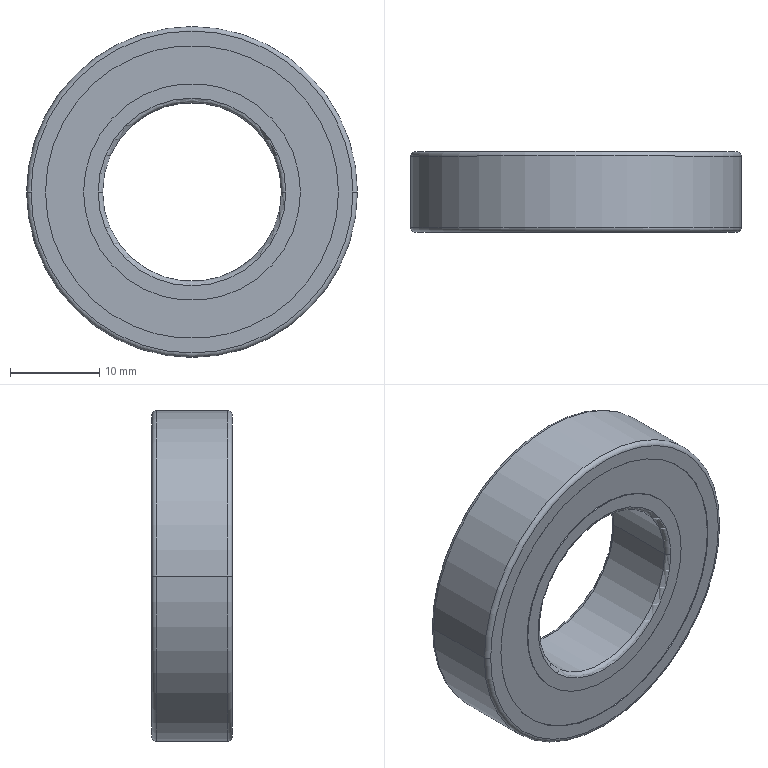Part | NX | 1 solid | 26 faces | box 37 x 9 x 37 mm | volume 6754 mm3 | cylinder 12 | torus 8 | plane 6 | commonest cylinder face diameters 24.25 x4 32.75 x4 20 x2 37 x2
STEP:
#1=CARTESIAN_POINT('',(-10.5,-4.5,0.));
#2=VERTEX_POINT('',#1);
#3=CARTESIAN_POINT('',(10.5,-4.5,0.));
#4=VERTEX_POINT('',#3);
#5=CARTESIAN_POINT('',(0.,-4.5,0.));
#6=DIRECTION('',(0.,1.,0.));
#7=DIRECTION('',(1.,0.,0.));
#8=AXIS2_PLACEMENT_3D('',#5,#6,#7);
#9=CIRCLE('',#8,10.5);
#10=EDGE_CURVE('',#2,#4,#9,.T.);
#11=ORIENTED_EDGE('',*,*,#10,.F.);
#12=CARTESIAN_POINT('',(-10.,-4.,0.));
#13=VERTEX_POINT('',#12);
#14=CARTESIAN_POINT('',(-10.5,-4.,0.));
#15=DIRECTION('',(0.,0.,1.));
#16=DIRECTION('',(-1.,0.,0.));
#17=AXIS2_PLACEMENT_3D('',#14,#15,#16);
#18=CIRCLE('',#17,0.5);
#19=EDGE_CURVE('',#2,#13,#18,.T.);
#20=ORIENTED_EDGE('',*,*,#19,.T.);
#21=CARTESIAN_POINT('',(10.,-4.,0.));
#22=VERTEX_POINT('',#21);
#23=CARTESIAN_POINT('',(0.,-4.,0.));
#24=DIRECTION('',(0.,-1.,0.));
#25=DIRECTION('',(1.,0.,0.));
#26=AXIS2_PLACEMENT_3D('',#23,#24,#25);
#27=CIRCLE('',#26,10.);
#28=EDGE_CURVE('',#22,#13,#27,.T.);
#29=ORIENTED_EDGE('',*,*,#28,.F.);
#30=CARTESIAN_POINT('',(10.5,-4.,0.));
#31=DIRECTION('',(0.,0.,-1.));
#32=DIRECTION('',(1.,0.,0.));
#33=AXIS2_PLACEMENT_3D('',#30,#31,#32);
#34=CIRCLE('',#33,0.5);
#35=EDGE_CURVE('',#4,#22,#34,.T.);
#36=ORIENTED_EDGE('',*,*,#35,.F.);
#37=EDGE_LOOP('',(#11,#20,#29,#36));
#38=FACE_BOUND('',#37,.T.);
#39=CARTESIAN_POINT('',(0.,-4.,0.));
#40=DIRECTION('',(0.,-1.,0.));
#41=DIRECTION('',(1.,0.,0.));
#42=AXIS2_PLACEMENT_3D('',#39,#40,#41);
#43=TOROIDAL_SURFACE('',#42,10.5,0.5);
#44=ADVANCED_FACE('',(#38),#43,.T.);
#45=CARTESIAN_POINT('',(18.,-4.5,0.));
#46=VERTEX_POINT('',#45);
#47=CARTESIAN_POINT('',(-18.,-4.5,0.));
#48=VERTEX_POINT('',#47);
#49=CARTESIAN_POINT('',(0.,-4.5,0.));
#50=DIRECTION('',(0.,-1.,0.));
#51=DIRECTION('',(-1.,0.,0.));
#52=AXIS2_PLACEMENT_3D('',#49,#50,#51);
#53=CIRCLE('',#52,18.);
#54=EDGE_CURVE('',#46,#48,#53,.T.);
#55=ORIENTED_EDGE('',*,*,#54,.F.);
#56=CARTESIAN_POINT('',(18.5,-4.,0.));
#57=VERTEX_POINT('',#56);
#58=CARTESIAN_POINT('',(18.,-4.,0.));
#59=DIRECTION('',(0.,0.,-1.));
#60=DIRECTION('',(1.,0.,0.));
#61=AXIS2_PLACEMENT_3D('',#58,#59,#60);
#62=CIRCLE('',#61,0.5);
#63=EDGE_CURVE('',#57,#46,#62,.T.);
#64=ORIENTED_EDGE('',*,*,#63,.F.);
#65=CARTESIAN_POINT('',(-18.5,-4.,0.));
#66=VERTEX_POINT('',#65);
#67=CARTESIAN_POINT('',(0.,-4.,0.));
#68=DIRECTION('',(0.,-1.,0.));
#69=DIRECTION('',(1.,0.,0.));
#70=AXIS2_PLACEMENT_3D('',#67,#68,#69);
#71=CIRCLE('',#70,18.5);
#72=EDGE_CURVE('',#57,#66,#71,.T.);
#73=ORIENTED_EDGE('',*,*,#72,.T.);
#74=CARTESIAN_POINT('',(-18.,-4.,0.));
#75=DIRECTION('',(0.,0.,1.));
#76=DIRECTION('',(-1.,0.,0.));
#77=AXIS2_PLACEMENT_3D('',#74,#75,#76);
#78=CIRCLE('',#77,0.5);
#79=EDGE_CURVE('',#66,#48,#78,.T.);
#80=ORIENTED_EDGE('',*,*,#79,.T.);
#81=EDGE_LOOP('',(#55,#64,#73,#80));
#82=FACE_BOUND('',#81,.T.);
#83=CARTESIAN_POINT('',(0.,-4.,0.));
#84=DIRECTION('',(0.,-1.,0.));
#85=DIRECTION('',(1.,0.,0.));
#86=AXIS2_PLACEMENT_3D('',#83,#84,#85);
#87=TOROIDAL_SURFACE('',#86,18.,0.5);
#88=ADVANCED_FACE('',(#82),#87,.T.);
#89=CARTESIAN_POINT('',(10.,4.,0.));
#90=VERTEX_POINT('',#89);
#91=CARTESIAN_POINT('',(-10.,4.,0.));
#92=VERTEX_POINT('',#91);
#93=CARTESIAN_POINT('',(0.,4.,0.));
#94=DIRECTION('',(0.,-1.,0.));
#95=DIRECTION('',(1.,0.,0.));
#96=AXIS2_PLACEMENT_3D('',#93,#94,#95);
#97=CIRCLE('',#96,10.);
#98=EDGE_CURVE('',#90,#92,#97,.T.);
#99=ORIENTED_EDGE('',*,*,#98,.F.);
#100=CARTESIAN_POINT('',(10.,-4.95,0.));
#101=DIRECTION('',(0.,1.,0.));
#102=VECTOR('',#101,1000.);
#103=LINE('',#100,#102);
#104=EDGE_CURVE('',#22,#90,#103,.T.);
#105=ORIENTED_EDGE('',*,*,#104,.F.);
#106=ORIENTED_EDGE('',*,*,#28,.T.);
#107=CARTESIAN_POINT('',(-10.,-4.95,0.));
#108=DIRECTION('',(0.,1.,0.));
#109=VECTOR('',#108,1000.);
#110=LINE('',#107,#109);
#111=EDGE_CURVE('',#13,#92,#110,.T.);
#112=ORIENTED_EDGE('',*,*,#111,.T.);
#113=EDGE_LOOP('',(#99,#105,#106,#112));
#114=FACE_BOUND('',#113,.T.);
#115=CARTESIAN_POINT('',(0.,-4.95,0.));
#116=DIRECTION('',(0.,1.,0.));
#117=DIRECTION('',(1.,0.,0.));
#118=AXIS2_PLACEMENT_3D('',#115,#116,#117);
#119=CYLINDRICAL_SURFACE('',#118,10.);
#120=ADVANCED_FACE('',(#114),#119,.F.);
#121=CARTESIAN_POINT('',(16.375,-4.4,0.));
#122=VERTEX_POINT('',#121);
#123=CARTESIAN_POINT('',(-16.375,-4.4,0.));
#124=VERTEX_POINT('',#123);
#125=CARTESIAN_POINT('',(0.,-4.4,0.));
#126=DIRECTION('',(0.,-1.,0.));
#127=DIRECTION('',(-1.,0.,0.));
#128=AXIS2_PLACEMENT_3D('',#125,#126,#127);
#129=CIRCLE('',#128,16.375);
#130=EDGE_CURVE('',#122,#124,#129,.T.);
#131=ORIENTED_EDGE('',*,*,#130,.F.);
#132=CARTESIAN_POINT('',(16.375,-4.5,0.));
#133=VERTEX_POINT('',#132);
#134=CARTESIAN_POINT('',(16.375,-4.95,0.));
#135=DIRECTION('',(0.,1.,0.));
#136=VECTOR('',#135,1000.);
#137=LINE('',#134,#136);
#138=EDGE_CURVE('',#133,#122,#137,.T.);
#139=ORIENTED_EDGE('',*,*,#138,.F.);
#140=CARTESIAN_POINT('',(-16.375,-4.5,0.));
#141=VERTEX_POINT('',#140);
#142=CARTESIAN_POINT('',(0.,-4.5,0.));
#143=DIRECTION('',(0.,1.,0.));
#144=DIRECTION('',(-1.,0.,0.));
#145=AXIS2_PLACEMENT_3D('',#142,#143,#144);
#146=CIRCLE('',#145,16.375);
#147=EDGE_CURVE('',#141,#133,#146,.T.);
#148=ORIENTED_EDGE('',*,*,#147,.F.);
#149=CARTESIAN_POINT('',(-16.375,-4.95,0.));
#150=DIRECTION('',(0.,1.,0.));
#151=VECTOR('',#150,1000.);
#152=LINE('',#149,#151);
#153=EDGE_CURVE('',#141,#124,#152,.T.);
#154=ORIENTED_EDGE('',*,*,#153,.T.);
#155=EDGE_LOOP('',(#131,#139,#148,#154));
#156=FACE_BOUND('',#155,.T.);
#157=CARTESIAN_POINT('',(0.,-4.95,0.));
#158=DIRECTION('',(0.,1.,0.));
#159=DIRECTION('',(1.,0.,0.));
#160=AXIS2_PLACEMENT_3D('',#157,#158,#159);
#161=CYLINDRICAL_SURFACE('',#160,16.375);
#162=ADVANCED_FACE('',(#156),#161,.F.);
#163=CARTESIAN_POINT('',(-10.5,4.5,0.));
#164=VERTEX_POINT('',#163);
#165=CARTESIAN_POINT('',(10.5,4.5,0.));
#166=VERTEX_POINT('',#165);
#167=CARTESIAN_POINT('',(0.,4.5,0.));
#168=DIRECTION('',(0.,-1.,0.));
#169=DIRECTION('',(-1.,0.,0.));
#170=AXIS2_PLACEMENT_3D('',#167,#168,#169);
#171=CIRCLE('',#170,10.5);
#172=EDGE_CURVE('',#164,#166,#171,.T.);
#173=ORIENTED_EDGE('',*,*,#172,.F.);
#174=CARTESIAN_POINT('',(-10.5,4.,0.));
#175=DIRECTION('',(0.,0.,1.));
#176=DIRECTION('',(-1.,0.,0.));
#177=AXIS2_PLACEMENT_3D('',#174,#175,#176);
#178=CIRCLE('',#177,0.5);
#179=EDGE_CURVE('',#164,#92,#178,.F.);
#180=ORIENTED_EDGE('',*,*,#179,.T.);
#181=CARTESIAN_POINT('',(0.,4.,0.));
#182=DIRECTION('',(0.,-1.,0.));
#183=DIRECTION('',(1.,0.,0.));
#184=AXIS2_PLACEMENT_3D('',#181,#182,#183);
#185=CIRCLE('',#184,10.);
#186=EDGE_CURVE('',#92,#90,#185,.T.);
#187=ORIENTED_EDGE('',*,*,#186,.T.);
#188=CARTESIAN_POINT('',(10.5,4.,0.));
#189=DIRECTION('',(0.,0.,-1.));
#190=DIRECTION('',(1.,0.,0.));
#191=AXIS2_PLACEMENT_3D('',#188,#189,#190);
#192=CIRCLE('',#191,0.5);
#193=EDGE_CURVE('',#166,#90,#192,.F.);
#194=ORIENTED_EDGE('',*,*,#193,.F.);
#195=EDGE_LOOP('',(#173,#180,#187,#194));
#196=FACE_BOUND('',#195,.T.);
#197=CARTESIAN_POINT('',(0.,4.,0.));
#198=DIRECTION('',(0.,-1.,0.));
#199=DIRECTION('',(1.,0.,0.));
#200=AXIS2_PLACEMENT_3D('',#197,#198,#199);
#201=TOROIDAL_SURFACE('',#200,10.5,0.5);
#202=ADVANCED_FACE('',(#196),#201,.T.);
#203=CARTESIAN_POINT('',(12.125,-4.4,0.));
#204=VERTEX_POINT('',#203);
#205=CARTESIAN_POINT('',(-12.125,-4.4,0.));
#206=VERTEX_POINT('',#205);
#207=CARTESIAN_POINT('',(0.,-4.4,0.));
#208=DIRECTION('',(0.,1.,0.));
#209=DIRECTION('',(-1.,0.,0.));
#210=AXIS2_PLACEMENT_3D('',#207,#208,#209);
#211=CIRCLE('',#210,12.125);
#212=EDGE_CURVE('',#204,#206,#211,.T.);
#213=ORIENTED_EDGE('',*,*,#212,.F.);
#214=CARTESIAN_POINT('',(12.125,-4.5,0.));
#215=VERTEX_POINT('',#214);
#216=CARTESIAN_POINT('',(12.125,-4.95,0.));
#217=DIRECTION('',(0.,1.,0.));
#218=VECTOR('',#217,1000.);
#219=LINE('',#216,#218);
#220=EDGE_CURVE('',#215,#204,#219,.T.);
#221=ORIENTED_EDGE('',*,*,#220,.F.);
#222=CARTESIAN_POINT('',(-12.125,-4.5,0.));
#223=VERTEX_POINT('',#222);
#224=CARTESIAN_POINT('',(0.,-4.5,0.));
#225=DIRECTION('',(0.,-1.,0.));
#226=DIRECTION('',(-1.,0.,0.));
#227=AXIS2_PLACEMENT_3D('',#224,#225,#226);
#228=CIRCLE('',#227,12.125);
#229=EDGE_CURVE('',#223,#215,#228,.T.);
#230=ORIENTED_EDGE('',*,*,#229,.F.);
#231=CARTESIAN_POINT('',(-12.125,-4.95,0.));
#232=DIRECTION('',(0.,1.,0.));
#233=VECTOR('',#232,1000.);
#234=LINE('',#231,#233);
#235=EDGE_CURVE('',#223,#206,#234,.T.);
#236=ORIENTED_EDGE('',*,*,#235,.T.);
#237=EDGE_LOOP('',(#213,#221,#230,#236));
#238=FACE_BOUND('',#237,.T.);
#239=CARTESIAN_POINT('',(0.,-4.95,0.));
#240=DIRECTION('',(0.,1.,0.));
#241=DIRECTION('',(1.,0.,0.));
#242=AXIS2_PLACEMENT_3D('',#239,#240,#241);
#243=CYLINDRICAL_SURFACE('',#242,12.125);
#244=ADVANCED_FACE('',(#238),#243,.T.);
#245=CARTESIAN_POINT('',(-12.125,4.5,0.));
#246=VERTEX_POINT('',#245);
#247=CARTESIAN_POINT('',(12.125,4.5,0.));
#248=VERTEX_POINT('',#247);
#249=CARTESIAN_POINT('',(0.,4.5,0.));
#250=DIRECTION('',(0.,1.,0.));
#251=DIRECTION('',(-1.,0.,0.));
#252=AXIS2_PLACEMENT_3D('',#249,#250,#251);
#253=CIRCLE('',#252,12.125);
#254=EDGE_CURVE('',#246,#248,#253,.T.);
#255=ORIENTED_EDGE('',*,*,#254,.T.);
#256=CARTESIAN_POINT('',(0.,4.5,0.));
#257=DIRECTION('',(0.,1.,0.));
#258=DIRECTION('',(-1.,0.,0.));
#259=AXIS2_PLACEMENT_3D('',#256,#257,#258);
#260=CIRCLE('',#259,12.125);
#261=EDGE_CURVE('',#248,#246,#260,.T.);
#262=ORIENTED_EDGE('',*,*,#261,.T.);
#263=EDGE_LOOP('',(#255,#262));
#264=FACE_BOUND('',#263,.T.);
#265=ORIENTED_EDGE('',*,*,#172,.T.);
#266=CARTESIAN_POINT('',(0.,4.5,0.));
#267=DIRECTION('',(0.,-1.,0.));
#268=DIRECTION('',(-1.,0.,0.));
#269=AXIS2_PLACEMENT_3D('',#266,#267,#268);
#270=CIRCLE('',#269,10.5);
#271=EDGE_CURVE('',#166,#164,#270,.T.);
#272=ORIENTED_EDGE('',*,*,#271,.T.);
#273=EDGE_LOOP('',(#265,#272));
#274=FACE_BOUND('',#273,.T.);
#275=CARTESIAN_POINT('',(0.,4.5,0.));
#276=DIRECTION('',(0.,-1.,0.));
#277=DIRECTION('',(0.,0.,-1.));
#278=AXIS2_PLACEMENT_3D('',#275,#276,#277);
#279=PLANE('',#278);
#280=ADVANCED_FACE('',(#264,#274),#279,.F.);
#281=CARTESIAN_POINT('',(-12.125,4.4,0.));
#282=VERTEX_POINT('',#281);
#283=CARTESIAN_POINT('',(12.125,4.4,0.));
#284=VERTEX_POINT('',#283);
#285=CARTESIAN_POINT('',(0.,4.4,0.));
#286=DIRECTION('',(0.,-1.,0.));
#287=DIRECTION('',(-1.,0.,0.));
#288=AXIS2_PLACEMENT_3D('',#285,#286,#287);
#289=CIRCLE('',#288,12.125);
#290=EDGE_CURVE('',#282,#284,#289,.T.);
#291=ORIENTED_EDGE('',*,*,#290,.F.);
#292=CARTESIAN_POINT('',(-12.125,-4.95,0.));
#293=DIRECTION('',(0.,1.,0.));
#294=VECTOR('',#293,1000.);
#295=LINE('',#292,#294);
#296=EDGE_CURVE('',#246,#282,#295,.F.);
#297=ORIENTED_EDGE('',*,*,#296,.F.);
#298=ORIENTED_EDGE('',*,*,#261,.F.);
#299=CARTESIAN_POINT('',(12.125,-4.95,0.));
#300=DIRECTION('',(0.,1.,0.));
#301=VECTOR('',#300,1000.);
#302=LINE('',#299,#301);
#303=EDGE_CURVE('',#248,#284,#302,.F.);
#304=ORIENTED_EDGE('',*,*,#303,.T.);
#305=EDGE_LOOP('',(#291,#297,#298,#304));
#306=FACE_BOUND('',#305,.T.);
#307=CARTESIAN_POINT('',(0.,-4.95,0.));
#308=DIRECTION('',(0.,1.,0.));
#309=DIRECTION('',(1.,0.,0.));
#310=AXIS2_PLACEMENT_3D('',#307,#308,#309);
#311=CYLINDRICAL_SURFACE('',#310,12.125);
#312=ADVANCED_FACE('',(#306),#311,.T.);
#313=CARTESIAN_POINT('',(0.,-4.5,0.));
#314=DIRECTION('',(0.,-1.,0.));
#315=DIRECTION('',(-1.,0.,0.));
#316=AXIS2_PLACEMENT_3D('',#313,#314,#315);
#317=CIRCLE('',#316,12.125);
#318=EDGE_CURVE('',#215,#223,#317,.T.);
#319=ORIENTED_EDGE('',*,*,#318,.T.);
#320=ORIENTED_EDGE('',*,*,#229,.T.);
#321=EDGE_LOOP('',(#319,#320));
#322=FACE_BOUND('',#321,.T.);
#323=ORIENTED_EDGE('',*,*,#10,.T.);
#324=CARTESIAN_POINT('',(0.,-4.5,0.));
#325=DIRECTION('',(0.,1.,0.));
#326=DIRECTION('',(1.,0.,0.));
#327=AXIS2_PLACEMENT_3D('',#324,#325,#326);
#328=CIRCLE('',#327,10.5);
#329=EDGE_CURVE('',#4,#2,#328,.T.);
#330=ORIENTED_EDGE('',*,*,#329,.T.);
#331=EDGE_LOOP('',(#323,#330));
#332=FACE_BOUND('',#331,.T.);
#333=CARTESIAN_POINT('',(0.,-4.5,0.));
#334=DIRECTION('',(0.,-1.,0.));
#335=DIRECTION('',(0.,0.,-1.));
#336=AXIS2_PLACEMENT_3D('',#333,#334,#335);
#337=PLANE('',#336);
#338=ADVANCED_FACE('',(#322,#332),#337,.T.);
#339=CARTESIAN_POINT('',(-16.375,4.4,0.));
#340=VERTEX_POINT('',#339);
#341=CARTESIAN_POINT('',(16.375,4.4,0.));
#342=VERTEX_POINT('',#341);
#343=CARTESIAN_POINT('',(0.,4.4,0.));
#344=DIRECTION('',(0.,1.,0.));
#345=DIRECTION('',(-1.,0.,0.));
#346=AXIS2_PLACEMENT_3D('',#343,#344,#345);
#347=CIRCLE('',#346,16.375);
#348=EDGE_CURVE('',#340,#342,#347,.T.);
#349=ORIENTED_EDGE('',*,*,#348,.T.);
#350=CARTESIAN_POINT('',(0.,4.4,0.));
#351=DIRECTION('',(0.,1.,0.));
#352=DIRECTION('',(-1.,0.,0.));
#353=AXIS2_PLACEMENT_3D('',#350,#351,#352);
#354=CIRCLE('',#353,16.375);
#355=EDGE_CURVE('',#342,#340,#354,.T.);
#356=ORIENTED_EDGE('',*,*,#355,.T.);
#357=EDGE_LOOP('',(#349,#356));
#358=FACE_BOUND('',#357,.T.);
#359=ORIENTED_EDGE('',*,*,#290,.T.);
#360=CARTESIAN_POINT('',(0.,4.4,0.));
#361=DIRECTION('',(0.,-1.,0.));
#362=DIRECTION('',(-1.,0.,0.));
#363=AXIS2_PLACEMENT_3D('',#360,#361,#362);
#364=CIRCLE('',#363,12.125);
#365=EDGE_CURVE('',#284,#282,#364,.T.);
#366=ORIENTED_EDGE('',*,*,#365,.T.);
#367=EDGE_LOOP('',(#359,#366));
#368=FACE_BOUND('',#367,.T.);
#369=CARTESIAN_POINT('',(0.,4.4,0.));
#370=DIRECTION('',(0.,-1.,0.));
#371=DIRECTION('',(0.,0.,-1.));
#372=AXIS2_PLACEMENT_3D('',#369,#370,#371);
#373=PLANE('',#372);
#374=ADVANCED_FACE('',(#358,#368),#373,.F.);
#375=ORIENTED_EDGE('',*,*,#348,.F.);
#376=CARTESIAN_POINT('',(-16.375,4.5,0.));
#377=VERTEX_POINT('',#376);
#378=CARTESIAN_POINT('',(-16.375,-4.95,0.));
#379=DIRECTION('',(0.,1.,0.));
#380=VECTOR('',#379,1000.);
#381=LINE('',#378,#380);
#382=EDGE_CURVE('',#340,#377,#381,.T.);
#383=ORIENTED_EDGE('',*,*,#382,.T.);
#384=CARTESIAN_POINT('',(16.375,4.5,0.));
#385=VERTEX_POINT('',#384);
#386=CARTESIAN_POINT('',(0.,4.5,0.));
#387=DIRECTION('',(0.,-1.,0.));
#388=DIRECTION('',(-1.,0.,0.));
#389=AXIS2_PLACEMENT_3D('',#386,#387,#388);
#390=CIRCLE('',#389,16.375);
#391=EDGE_CURVE('',#385,#377,#390,.T.);
#392=ORIENTED_EDGE('',*,*,#391,.F.);
#393=CARTESIAN_POINT('',(16.375,-4.95,0.));
#394=DIRECTION('',(0.,1.,0.));
#395=VECTOR('',#394,1000.);
#396=LINE('',#393,#395);
#397=EDGE_CURVE('',#342,#385,#396,.T.);
#398=ORIENTED_EDGE('',*,*,#397,.F.);
#399=EDGE_LOOP('',(#375,#383,#392,#398));
#400=FACE_BOUND('',#399,.T.);
#401=CARTESIAN_POINT('',(0.,-4.95,0.));
#402=DIRECTION('',(0.,1.,0.));
#403=DIRECTION('',(1.,0.,0.));
#404=AXIS2_PLACEMENT_3D('',#401,#402,#403);
#405=CYLINDRICAL_SURFACE('',#404,16.375);
#406=ADVANCED_FACE('',(#400),#405,.F.);
#407=ORIENTED_EDGE('',*,*,#130,.T.);
#408=CARTESIAN_POINT('',(0.,-4.4,0.));
#409=DIRECTION('',(0.,-1.,0.));
#410=DIRECTION('',(-1.,0.,0.));
#411=AXIS2_PLACEMENT_3D('',#408,#409,#410);
#412=CIRCLE('',#411,16.375);
#413=EDGE_CURVE('',#124,#122,#412,.T.);
#414=ORIENTED_EDGE('',*,*,#413,.T.);
#415=EDGE_LOOP('',(#407,#414));
#416=FACE_BOUND('',#415,.T.);
#417=ORIENTED_EDGE('',*,*,#212,.T.);
#418=CARTESIAN_POINT('',(0.,-4.4,0.));
#419=DIRECTION('',(0.,1.,0.));
#420=DIRECTION('',(-1.,0.,0.));
#421=AXIS2_PLACEMENT_3D('',#418,#419,#420);
#422=CIRCLE('',#421,12.125);
#423=EDGE_CURVE('',#206,#204,#422,.T.);
#424=ORIENTED_EDGE('',*,*,#423,.T.);
#425=EDGE_LOOP('',(#417,#424));
#426=FACE_BOUND('',#425,.T.);
#427=CARTESIAN_POINT('',(0.,-4.4,0.));
#428=DIRECTION('',(0.,-1.,0.));
#429=DIRECTION('',(0.,0.,-1.));
#430=AXIS2_PLACEMENT_3D('',#427,#428,#429);
#431=PLANE('',#430);
#432=ADVANCED_FACE('',(#416,#426),#431,.T.);
#433=CARTESIAN_POINT('',(-18.,4.5,0.));
#434=VERTEX_POINT('',#433);
#435=CARTESIAN_POINT('',(18.,4.5,0.));
#436=VERTEX_POINT('',#435);
#437=CARTESIAN_POINT('',(0.,4.5,0.));
#438=DIRECTION('',(0.,1.,0.));
#439=DIRECTION('',(-1.,0.,0.));
#440=AXIS2_PLACEMENT_3D('',#437,#438,#439);
#441=CIRCLE('',#440,18.);
#442=EDGE_CURVE('',#434,#436,#441,.T.);
#443=ORIENTED_EDGE('',*,*,#442,.T.);
#444=CARTESIAN_POINT('',(0.,4.5,0.));
#445=DIRECTION('',(0.,1.,0.));
#446=DIRECTION('',(-1.,0.,0.));
#447=AXIS2_PLACEMENT_3D('',#444,#445,#446);
#448=CIRCLE('',#447,18.);
#449=EDGE_CURVE('',#436,#434,#448,.T.);
#450=ORIENTED_EDGE('',*,*,#449,.T.);
#451=EDGE_LOOP('',(#443,#450));
#452=FACE_BOUND('',#451,.T.);
#453=ORIENTED_EDGE('',*,*,#391,.T.);
#454=CARTESIAN_POINT('',(0.,4.5,0.));
#455=DIRECTION('',(0.,-1.,0.));
#456=DIRECTION('',(-1.,0.,0.));
#457=AXIS2_PLACEMENT_3D('',#454,#455,#456);
#458=CIRCLE('',#457,16.375);
#459=EDGE_CURVE('',#377,#385,#458,.T.);
#460=ORIENTED_EDGE('',*,*,#459,.T.);
#461=EDGE_LOOP('',(#453,#460));
#462=FACE_BOUND('',#461,.T.);
#463=CARTESIAN_POINT('',(0.,4.5,0.));
#464=DIRECTION('',(0.,-1.,0.));
#465=DIRECTION('',(0.,0.,-1.));
#466=AXIS2_PLACEMENT_3D('',#463,#464,#465);
#467=PLANE('',#466);
#468=ADVANCED_FACE('',(#452,#462),#467,.F.);
#469=CARTESIAN_POINT('',(-18.5,4.,0.));
#470=VERTEX_POINT('',#469);
#471=CARTESIAN_POINT('',(18.5,4.,0.));
#472=VERTEX_POINT('',#471);
#473=CARTESIAN_POINT('',(0.,4.,0.));
#474=DIRECTION('',(0.,-1.,0.));
#475=DIRECTION('',(1.,0.,0.));
#476=AXIS2_PLACEMENT_3D('',#473,#474,#475);
#477=CIRCLE('',#476,18.5);
#478=EDGE_CURVE('',#470,#472,#477,.T.);
#479=ORIENTED_EDGE('',*,*,#478,.F.);
#480=CARTESIAN_POINT('',(-18.,4.,0.));
#481=DIRECTION('',(0.,0.,1.));
#482=DIRECTION('',(-1.,0.,0.));
#483=AXIS2_PLACEMENT_3D('',#480,#481,#482);
#484=CIRCLE('',#483,0.5);
#485=EDGE_CURVE('',#470,#434,#484,.F.);
#486=ORIENTED_EDGE('',*,*,#485,.T.);
#487=ORIENTED_EDGE('',*,*,#449,.F.);
#488=CARTESIAN_POINT('',(18.,4.,0.));
#489=DIRECTION('',(0.,0.,-1.));
#490=DIRECTION('',(1.,0.,0.));
#491=AXIS2_PLACEMENT_3D('',#488,#489,#490);
#492=CIRCLE('',#491,0.5);
#493=EDGE_CURVE('',#472,#436,#492,.F.);
#494=ORIENTED_EDGE('',*,*,#493,.F.);
#495=EDGE_LOOP('',(#479,#486,#487,#494));
#496=FACE_BOUND('',#495,.T.);
#497=CARTESIAN_POINT('',(0.,4.,0.));
#498=DIRECTION('',(0.,-1.,0.));
#499=DIRECTION('',(1.,0.,0.));
#500=AXIS2_PLACEMENT_3D('',#497,#498,#499);
#501=TOROIDAL_SURFACE('',#500,18.,0.5);
#502=ADVANCED_FACE('',(#496),#501,.T.);
#503=ORIENTED_EDGE('',*,*,#54,.T.);
#504=CARTESIAN_POINT('',(0.,-4.5,0.));
#505=DIRECTION('',(0.,-1.,0.));
#506=DIRECTION('',(-1.,0.,0.));
#507=AXIS2_PLACEMENT_3D('',#504,#505,#506);
#508=CIRCLE('',#507,18.);
#509=EDGE_CURVE('',#48,#46,#508,.T.);
#510=ORIENTED_EDGE('',*,*,#509,.T.);
#511=EDGE_LOOP('',(#503,#510));
#512=FACE_BOUND('',#511,.T.);
#513=CARTESIAN_POINT('',(0.,-4.5,0.));
#514=DIRECTION('',(0.,1.,0.));
#515=DIRECTION('',(-1.,0.,0.));
#516=AXIS2_PLACEMENT_3D('',#513,#514,#515);
#517=CIRCLE('',#516,16.375);
#518=EDGE_CURVE('',#133,#141,#517,.T.);
#519=ORIENTED_EDGE('',*,*,#518,.T.);
#520=ORIENTED_EDGE('',*,*,#147,.T.);
#521=EDGE_LOOP('',(#519,#520));
#522=FACE_BOUND('',#521,.T.);
#523=CARTESIAN_POINT('',(0.,-4.5,0.));
#524=DIRECTION('',(0.,-1.,0.));
#525=DIRECTION('',(0.,0.,-1.));
#526=AXIS2_PLACEMENT_3D('',#523,#524,#525);
#527=PLANE('',#526);
#528=ADVANCED_FACE('',(#512,#522),#527,.T.);
#529=ORIENTED_EDGE('',*,*,#72,.F.);
#530=CARTESIAN_POINT('',(18.5,-4.95,0.));
#531=DIRECTION('',(0.,1.,0.));
#532=VECTOR('',#531,1000.);
#533=LINE('',#530,#532);
#534=EDGE_CURVE('',#57,#472,#533,.T.);
#535=ORIENTED_EDGE('',*,*,#534,.T.);
#536=CARTESIAN_POINT('',(0.,4.,0.));
#537=DIRECTION('',(0.,-1.,0.));
#538=DIRECTION('',(1.,0.,0.));
#539=AXIS2_PLACEMENT_3D('',#536,#537,#538);
#540=CIRCLE('',#539,18.5);
#541=EDGE_CURVE('',#472,#470,#540,.T.);
#542=ORIENTED_EDGE('',*,*,#541,.T.);
#543=CARTESIAN_POINT('',(-18.5,-4.95,0.));
#544=DIRECTION('',(0.,1.,0.));
#545=VECTOR('',#544,1000.);
#546=LINE('',#543,#545);
#547=EDGE_CURVE('',#66,#470,#546,.T.);
#548=ORIENTED_EDGE('',*,*,#547,.F.);
#549=EDGE_LOOP('',(#529,#535,#542,#548));
#550=FACE_BOUND('',#549,.T.);
#551=CARTESIAN_POINT('',(0.,-4.95,0.));
#552=DIRECTION('',(0.,1.,0.));
#553=DIRECTION('',(1.,0.,0.));
#554=AXIS2_PLACEMENT_3D('',#551,#552,#553);
#555=CYLINDRICAL_SURFACE('',#554,18.5);
#556=ADVANCED_FACE('',(#550),#555,.T.);
#557=ORIENTED_EDGE('',*,*,#397,.T.);
#558=ORIENTED_EDGE('',*,*,#459,.F.);
#559=ORIENTED_EDGE('',*,*,#382,.F.);
#560=ORIENTED_EDGE('',*,*,#355,.F.);
#561=EDGE_LOOP('',(#557,#558,#559,#560));
#562=FACE_BOUND('',#561,.T.);
#563=CARTESIAN_POINT('',(0.,-4.95,0.));
#564=DIRECTION('',(0.,1.,0.));
#565=DIRECTION('',(1.,0.,0.));
#566=AXIS2_PLACEMENT_3D('',#563,#564,#565);
#567=CYLINDRICAL_SURFACE('',#566,16.375);
#568=ADVANCED_FACE('',(#562),#567,.F.);
#569=ORIENTED_EDGE('',*,*,#104,.T.);
#570=ORIENTED_EDGE('',*,*,#186,.F.);
#571=ORIENTED_EDGE('',*,*,#111,.F.);
#572=CARTESIAN_POINT('',(0.,-4.,0.));
#573=DIRECTION('',(0.,-1.,0.));
#574=DIRECTION('',(1.,0.,0.));
#575=AXIS2_PLACEMENT_3D('',#572,#573,#574);
#576=CIRCLE('',#575,10.);
#577=EDGE_CURVE('',#13,#22,#576,.T.);
#578=ORIENTED_EDGE('',*,*,#577,.T.);
#579=EDGE_LOOP('',(#569,#570,#571,#578));
#580=FACE_BOUND('',#579,.T.);
#581=CARTESIAN_POINT('',(0.,-4.95,0.));
#582=DIRECTION('',(0.,1.,0.));
#583=DIRECTION('',(1.,0.,0.));
#584=AXIS2_PLACEMENT_3D('',#581,#582,#583);
#585=CYLINDRICAL_SURFACE('',#584,10.);
#586=ADVANCED_FACE('',(#580),#585,.F.);
#587=ORIENTED_EDGE('',*,*,#478,.T.);
#588=ORIENTED_EDGE('',*,*,#534,.F.);
#589=CARTESIAN_POINT('',(0.,-4.,0.));
#590=DIRECTION('',(0.,-1.,0.));
#591=DIRECTION('',(1.,0.,0.));
#592=AXIS2_PLACEMENT_3D('',#589,#590,#591);
#593=CIRCLE('',#592,18.5);
#594=EDGE_CURVE('',#66,#57,#593,.T.);
#595=ORIENTED_EDGE('',*,*,#594,.F.);
#596=ORIENTED_EDGE('',*,*,#547,.T.);
#597=EDGE_LOOP('',(#587,#588,#595,#596));
#598=FACE_BOUND('',#597,.T.);
#599=CARTESIAN_POINT('',(0.,-4.95,0.));
#600=DIRECTION('',(0.,1.,0.));
#601=DIRECTION('',(1.,0.,0.));
#602=AXIS2_PLACEMENT_3D('',#599,#600,#601);
#603=CYLINDRICAL_SURFACE('',#602,18.5);
#604=ADVANCED_FACE('',(#598),#603,.T.);
#605=ORIENTED_EDGE('',*,*,#518,.F.);
#606=ORIENTED_EDGE('',*,*,#138,.T.);
#607=ORIENTED_EDGE('',*,*,#413,.F.);
#608=ORIENTED_EDGE('',*,*,#153,.F.);
#609=EDGE_LOOP('',(#605,#606,#607,#608));
#610=FACE_BOUND('',#609,.T.);
#611=CARTESIAN_POINT('',(0.,-4.95,0.));
#612=DIRECTION('',(0.,1.,0.));
#613=DIRECTION('',(1.,0.,0.));
#614=AXIS2_PLACEMENT_3D('',#611,#612,#613);
#615=CYLINDRICAL_SURFACE('',#614,16.375);
#616=ADVANCED_FACE('',(#610),#615,.F.);
#617=ORIENTED_EDGE('',*,*,#254,.F.);
#618=ORIENTED_EDGE('',*,*,#296,.T.);
#619=ORIENTED_EDGE('',*,*,#365,.F.);
#620=ORIENTED_EDGE('',*,*,#303,.F.);
#621=EDGE_LOOP('',(#617,#618,#619,#620));
#622=FACE_BOUND('',#621,.T.);
#623=CARTESIAN_POINT('',(0.,-4.95,0.));
#624=DIRECTION('',(0.,1.,0.));
#625=DIRECTION('',(1.,0.,0.));
#626=AXIS2_PLACEMENT_3D('',#623,#624,#625);
#627=CYLINDRICAL_SURFACE('',#626,12.125);
#628=ADVANCED_FACE('',(#622),#627,.T.);
#629=ORIENTED_EDGE('',*,*,#318,.F.);
#630=ORIENTED_EDGE('',*,*,#220,.T.);
#631=ORIENTED_EDGE('',*,*,#423,.F.);
#632=ORIENTED_EDGE('',*,*,#235,.F.);
#633=EDGE_LOOP('',(#629,#630,#631,#632));
#634=FACE_BOUND('',#633,.T.);
#635=CARTESIAN_POINT('',(0.,-4.95,0.));
#636=DIRECTION('',(0.,1.,0.));
#637=DIRECTION('',(1.,0.,0.));
#638=AXIS2_PLACEMENT_3D('',#635,#636,#637);
#639=CYLINDRICAL_SURFACE('',#638,12.125);
#640=ADVANCED_FACE('',(#634),#639,.T.);
#641=ORIENTED_EDGE('',*,*,#35,.T.);
#642=ORIENTED_EDGE('',*,*,#577,.F.);
#643=ORIENTED_EDGE('',*,*,#19,.F.);
#644=ORIENTED_EDGE('',*,*,#329,.F.);
#645=EDGE_LOOP('',(#641,#642,#643,#644));
#646=FACE_BOUND('',#645,.T.);
#647=CARTESIAN_POINT('',(0.,-4.,0.));
#648=DIRECTION('',(0.,-1.,0.));
#649=DIRECTION('',(1.,0.,0.));
#650=AXIS2_PLACEMENT_3D('',#647,#648,#649);
#651=TOROIDAL_SURFACE('',#650,10.5,0.5);
#652=ADVANCED_FACE('',(#646),#651,.T.);
#653=ORIENTED_EDGE('',*,*,#442,.F.);
#654=ORIENTED_EDGE('',*,*,#485,.F.);
#655=ORIENTED_EDGE('',*,*,#541,.F.);
#656=ORIENTED_EDGE('',*,*,#493,.T.);
#657=EDGE_LOOP('',(#653,#654,#655,#656));
#658=FACE_BOUND('',#657,.T.);
#659=CARTESIAN_POINT('',(0.,4.,0.));
#660=DIRECTION('',(0.,-1.,0.));
#661=DIRECTION('',(1.,0.,0.));
#662=AXIS2_PLACEMENT_3D('',#659,#660,#661);
#663=TOROIDAL_SURFACE('',#662,18.,0.5);
#664=ADVANCED_FACE('',(#658),#663,.T.);
#665=ORIENTED_EDGE('',*,*,#63,.T.);
#666=ORIENTED_EDGE('',*,*,#509,.F.);
#667=ORIENTED_EDGE('',*,*,#79,.F.);
#668=ORIENTED_EDGE('',*,*,#594,.T.);
#669=EDGE_LOOP('',(#665,#666,#667,#668));
#670=FACE_BOUND('',#669,.T.);
#671=CARTESIAN_POINT('',(0.,-4.,0.));
#672=DIRECTION('',(0.,-1.,0.));
#673=DIRECTION('',(1.,0.,0.));
#674=AXIS2_PLACEMENT_3D('',#671,#672,#673);
#675=TOROIDAL_SURFACE('',#674,18.,0.5);
#676=ADVANCED_FACE('',(#670),#675,.T.);
#677=ORIENTED_EDGE('',*,*,#98,.T.);
#678=ORIENTED_EDGE('',*,*,#179,.F.);
#679=ORIENTED_EDGE('',*,*,#271,.F.);
#680=ORIENTED_EDGE('',*,*,#193,.T.);
#681=EDGE_LOOP('',(#677,#678,#679,#680));
#682=FACE_BOUND('',#681,.T.);
#683=CARTESIAN_POINT('',(0.,4.,0.));
#684=DIRECTION('',(0.,-1.,0.));
#685=DIRECTION('',(1.,0.,0.));
#686=AXIS2_PLACEMENT_3D('',#683,#684,#685);
#687=TOROIDAL_SURFACE('',#686,10.5,0.5);
#688=ADVANCED_FACE('',(#682),#687,.T.);
#689=CLOSED_SHELL('',(#44,#88,#120,#162,#202,#244,#280,#312,#338,#374,#406,#432,#468,#502,#528,#556,#568,#586,#604,#616,#628,#640,#652,#664,#676,#688));
#690=MANIFOLD_SOLID_BREP('',#689);
#691=(LENGTH_UNIT()NAMED_UNIT(*)SI_UNIT(.MILLI.,.METRE.));
#692=UNCERTAINTY_MEASURE_WITH_UNIT(LENGTH_MEASURE(0.00001),#691,'','');
#693=(NAMED_UNIT(*)PLANE_ANGLE_UNIT()SI_UNIT($,.RADIAN.));
#694=(NAMED_UNIT(*)SI_UNIT($,.STERADIAN.)SOLID_ANGLE_UNIT());
#695=(GEOMETRIC_REPRESENTATION_CONTEXT(3)GLOBAL_UNCERTAINTY_ASSIGNED_CONTEXT((#692))GLOBAL_UNIT_ASSIGNED_CONTEXT((#691,#693,#694))REPRESENTATION_CONTEXT('',''));
#696=ADVANCED_BREP_SHAPE_REPRESENTATION('',(#690),#695);